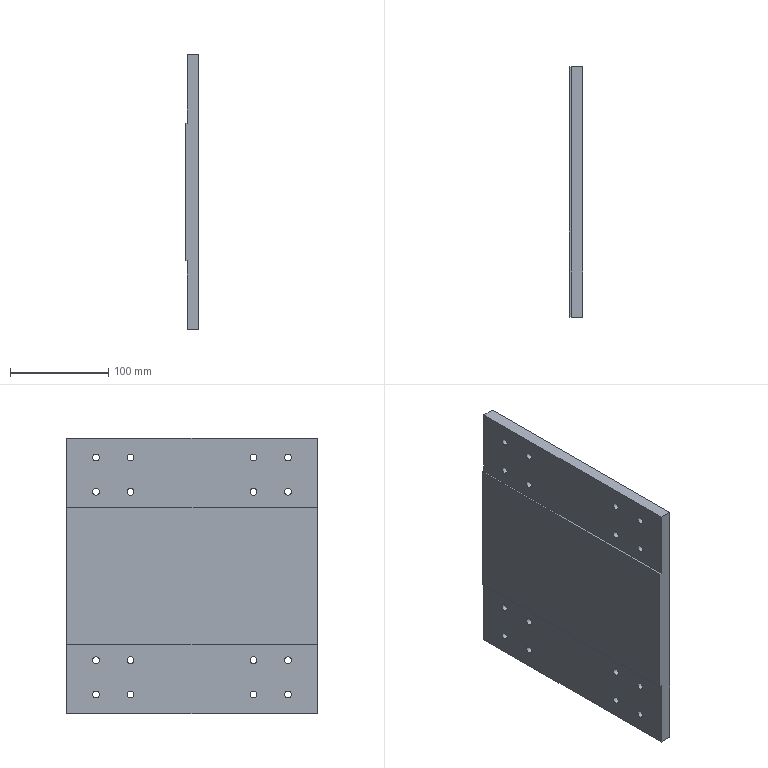Part | SolidWorks | features Extrusion 1, ICE 1 | 1 solid | 42 faces | box 14 x 255 x 280 mm | volume 920811 mm3 | cylinder 32 | plane 10 | commonest cylinder face diameters 7 x32
STEP:
#1=CARTESIAN_POINT('',(14.,62.5,-82.));
#2=VERTEX_POINT('',#1);
#3=CARTESIAN_POINT('',(14.,62.5,-89.));
#4=VERTEX_POINT('',#3);
#5=CARTESIAN_POINT('',(14.,62.5,-85.5));
#6=DIRECTION('',(1.,0.,0.));
#7=DIRECTION('',(0.,0.,-1.));
#8=AXIS2_PLACEMENT_3D('',#5,#6,#7);
#9=CIRCLE('',#8,3.5);
#10=EDGE_CURVE('',#2,#4,#9,.T.);
#11=ORIENTED_EDGE('',*,*,#10,.T.);
#12=CARTESIAN_POINT('',(2.,62.5,-89.));
#13=VERTEX_POINT('',#12);
#14=CARTESIAN_POINT('',(14.,62.5,-89.));
#15=DIRECTION('',(-1.,0.,0.));
#16=VECTOR('',#15,1000.);
#17=LINE('',#14,#16);
#18=EDGE_CURVE('',#4,#13,#17,.T.);
#19=ORIENTED_EDGE('',*,*,#18,.T.);
#20=CARTESIAN_POINT('',(2.,62.5,-82.));
#21=VERTEX_POINT('',#20);
#22=CARTESIAN_POINT('',(2.,62.5,-85.5));
#23=DIRECTION('',(-1.,0.,0.));
#24=DIRECTION('',(0.,0.,1.));
#25=AXIS2_PLACEMENT_3D('',#22,#23,#24);
#26=CIRCLE('',#25,3.5);
#27=EDGE_CURVE('',#13,#21,#26,.T.);
#28=ORIENTED_EDGE('',*,*,#27,.T.);
#29=CARTESIAN_POINT('',(14.,62.5,-82.));
#30=DIRECTION('',(-1.,0.,0.));
#31=VECTOR('',#30,1000.);
#32=LINE('',#29,#31);
#33=EDGE_CURVE('',#2,#21,#32,.T.);
#34=ORIENTED_EDGE('',*,*,#33,.F.);
#35=EDGE_LOOP('',(#11,#19,#28,#34));
#36=FACE_OUTER_BOUND('',#35,.T.);
#37=CARTESIAN_POINT('',(14.,62.5,-85.5));
#38=DIRECTION('',(-1.,0.,0.));
#39=DIRECTION('',(0.,0.,1.));
#40=AXIS2_PLACEMENT_3D('',#37,#38,#39);
#41=CYLINDRICAL_SURFACE('',#40,3.5);
#42=ADVANCED_FACE('',(#36),#41,.F.);
#43=CARTESIAN_POINT('',(14.,62.5,-117.));
#44=VERTEX_POINT('',#43);
#45=CARTESIAN_POINT('',(14.,62.5,-124.));
#46=VERTEX_POINT('',#45);
#47=CARTESIAN_POINT('',(14.,62.5,-120.5));
#48=DIRECTION('',(1.,0.,0.));
#49=DIRECTION('',(0.,0.,-1.));
#50=AXIS2_PLACEMENT_3D('',#47,#48,#49);
#51=CIRCLE('',#50,3.5);
#52=EDGE_CURVE('',#44,#46,#51,.T.);
#53=ORIENTED_EDGE('',*,*,#52,.T.);
#54=CARTESIAN_POINT('',(2.,62.5,-124.));
#55=VERTEX_POINT('',#54);
#56=CARTESIAN_POINT('',(14.,62.5,-124.));
#57=DIRECTION('',(-1.,0.,0.));
#58=VECTOR('',#57,1000.);
#59=LINE('',#56,#58);
#60=EDGE_CURVE('',#46,#55,#59,.T.);
#61=ORIENTED_EDGE('',*,*,#60,.T.);
#62=CARTESIAN_POINT('',(2.,62.5,-117.));
#63=VERTEX_POINT('',#62);
#64=CARTESIAN_POINT('',(2.,62.5,-120.5));
#65=DIRECTION('',(-1.,0.,0.));
#66=DIRECTION('',(0.,0.,1.));
#67=AXIS2_PLACEMENT_3D('',#64,#65,#66);
#68=CIRCLE('',#67,3.5);
#69=EDGE_CURVE('',#55,#63,#68,.T.);
#70=ORIENTED_EDGE('',*,*,#69,.T.);
#71=CARTESIAN_POINT('',(14.,62.5,-117.));
#72=DIRECTION('',(-1.,0.,0.));
#73=VECTOR('',#72,1000.);
#74=LINE('',#71,#73);
#75=EDGE_CURVE('',#44,#63,#74,.T.);
#76=ORIENTED_EDGE('',*,*,#75,.F.);
#77=EDGE_LOOP('',(#53,#61,#70,#76));
#78=FACE_OUTER_BOUND('',#77,.T.);
#79=CARTESIAN_POINT('',(14.,62.5,-120.5));
#80=DIRECTION('',(-1.,0.,0.));
#81=DIRECTION('',(0.,0.,1.));
#82=AXIS2_PLACEMENT_3D('',#79,#80,#81);
#83=CYLINDRICAL_SURFACE('',#82,3.5);
#84=ADVANCED_FACE('',(#78),#83,.F.);
#85=CARTESIAN_POINT('',(14.,-97.5,-117.));
#86=VERTEX_POINT('',#85);
#87=CARTESIAN_POINT('',(14.,-97.5,-124.));
#88=VERTEX_POINT('',#87);
#89=CARTESIAN_POINT('',(14.,-97.5,-120.5));
#90=DIRECTION('',(1.,0.,0.));
#91=DIRECTION('',(0.,0.,-1.));
#92=AXIS2_PLACEMENT_3D('',#89,#90,#91);
#93=CIRCLE('',#92,3.5);
#94=EDGE_CURVE('',#86,#88,#93,.T.);
#95=ORIENTED_EDGE('',*,*,#94,.T.);
#96=CARTESIAN_POINT('',(2.,-97.5,-124.));
#97=VERTEX_POINT('',#96);
#98=CARTESIAN_POINT('',(14.,-97.5,-124.));
#99=DIRECTION('',(-1.,0.,0.));
#100=VECTOR('',#99,1000.);
#101=LINE('',#98,#100);
#102=EDGE_CURVE('',#88,#97,#101,.T.);
#103=ORIENTED_EDGE('',*,*,#102,.T.);
#104=CARTESIAN_POINT('',(2.,-97.5,-117.));
#105=VERTEX_POINT('',#104);
#106=CARTESIAN_POINT('',(2.,-97.5,-120.5));
#107=DIRECTION('',(-1.,0.,0.));
#108=DIRECTION('',(0.,0.,1.));
#109=AXIS2_PLACEMENT_3D('',#106,#107,#108);
#110=CIRCLE('',#109,3.5);
#111=EDGE_CURVE('',#97,#105,#110,.T.);
#112=ORIENTED_EDGE('',*,*,#111,.T.);
#113=CARTESIAN_POINT('',(14.,-97.5,-117.));
#114=DIRECTION('',(-1.,0.,0.));
#115=VECTOR('',#114,1000.);
#116=LINE('',#113,#115);
#117=EDGE_CURVE('',#86,#105,#116,.T.);
#118=ORIENTED_EDGE('',*,*,#117,.F.);
#119=EDGE_LOOP('',(#95,#103,#112,#118));
#120=FACE_OUTER_BOUND('',#119,.T.);
#121=CARTESIAN_POINT('',(14.,-97.5,-120.5));
#122=DIRECTION('',(-1.,0.,0.));
#123=DIRECTION('',(0.,0.,1.));
#124=AXIS2_PLACEMENT_3D('',#121,#122,#123);
#125=CYLINDRICAL_SURFACE('',#124,3.5);
#126=ADVANCED_FACE('',(#120),#125,.F.);
#127=CARTESIAN_POINT('',(14.,-97.5,-82.));
#128=VERTEX_POINT('',#127);
#129=CARTESIAN_POINT('',(14.,-97.5,-89.));
#130=VERTEX_POINT('',#129);
#131=CARTESIAN_POINT('',(14.,-97.5,-85.5));
#132=DIRECTION('',(1.,0.,0.));
#133=DIRECTION('',(0.,0.,-1.));
#134=AXIS2_PLACEMENT_3D('',#131,#132,#133);
#135=CIRCLE('',#134,3.5);
#136=EDGE_CURVE('',#128,#130,#135,.T.);
#137=ORIENTED_EDGE('',*,*,#136,.T.);
#138=CARTESIAN_POINT('',(2.,-97.5,-89.));
#139=VERTEX_POINT('',#138);
#140=CARTESIAN_POINT('',(14.,-97.5,-89.));
#141=DIRECTION('',(-1.,0.,0.));
#142=VECTOR('',#141,1000.);
#143=LINE('',#140,#142);
#144=EDGE_CURVE('',#130,#139,#143,.T.);
#145=ORIENTED_EDGE('',*,*,#144,.T.);
#146=CARTESIAN_POINT('',(2.,-97.5,-82.));
#147=VERTEX_POINT('',#146);
#148=CARTESIAN_POINT('',(2.,-97.5,-85.5));
#149=DIRECTION('',(-1.,0.,0.));
#150=DIRECTION('',(0.,0.,1.));
#151=AXIS2_PLACEMENT_3D('',#148,#149,#150);
#152=CIRCLE('',#151,3.5);
#153=EDGE_CURVE('',#139,#147,#152,.T.);
#154=ORIENTED_EDGE('',*,*,#153,.T.);
#155=CARTESIAN_POINT('',(14.,-97.5,-82.));
#156=DIRECTION('',(-1.,0.,0.));
#157=VECTOR('',#156,1000.);
#158=LINE('',#155,#157);
#159=EDGE_CURVE('',#128,#147,#158,.T.);
#160=ORIENTED_EDGE('',*,*,#159,.F.);
#161=EDGE_LOOP('',(#137,#145,#154,#160));
#162=FACE_OUTER_BOUND('',#161,.T.);
#163=CARTESIAN_POINT('',(14.,-97.5,-85.5));
#164=DIRECTION('',(-1.,0.,0.));
#165=DIRECTION('',(0.,0.,1.));
#166=AXIS2_PLACEMENT_3D('',#163,#164,#165);
#167=CYLINDRICAL_SURFACE('',#166,3.5);
#168=ADVANCED_FACE('',(#162),#167,.F.);
#169=CARTESIAN_POINT('',(14.,-62.5,-117.));
#170=VERTEX_POINT('',#169);
#171=CARTESIAN_POINT('',(14.,-62.5,-124.));
#172=VERTEX_POINT('',#171);
#173=CARTESIAN_POINT('',(14.,-62.5,-120.5));
#174=DIRECTION('',(1.,0.,0.));
#175=DIRECTION('',(0.,0.,-1.));
#176=AXIS2_PLACEMENT_3D('',#173,#174,#175);
#177=CIRCLE('',#176,3.5);
#178=EDGE_CURVE('',#170,#172,#177,.T.);
#179=ORIENTED_EDGE('',*,*,#178,.T.);
#180=CARTESIAN_POINT('',(2.,-62.5,-124.));
#181=VERTEX_POINT('',#180);
#182=CARTESIAN_POINT('',(14.,-62.5,-124.));
#183=DIRECTION('',(-1.,0.,0.));
#184=VECTOR('',#183,1000.);
#185=LINE('',#182,#184);
#186=EDGE_CURVE('',#172,#181,#185,.T.);
#187=ORIENTED_EDGE('',*,*,#186,.T.);
#188=CARTESIAN_POINT('',(2.,-62.5,-117.));
#189=VERTEX_POINT('',#188);
#190=CARTESIAN_POINT('',(2.,-62.5,-120.5));
#191=DIRECTION('',(-1.,0.,0.));
#192=DIRECTION('',(0.,0.,1.));
#193=AXIS2_PLACEMENT_3D('',#190,#191,#192);
#194=CIRCLE('',#193,3.5);
#195=EDGE_CURVE('',#181,#189,#194,.T.);
#196=ORIENTED_EDGE('',*,*,#195,.T.);
#197=CARTESIAN_POINT('',(14.,-62.5,-117.));
#198=DIRECTION('',(-1.,0.,0.));
#199=VECTOR('',#198,1000.);
#200=LINE('',#197,#199);
#201=EDGE_CURVE('',#170,#189,#200,.T.);
#202=ORIENTED_EDGE('',*,*,#201,.F.);
#203=EDGE_LOOP('',(#179,#187,#196,#202));
#204=FACE_OUTER_BOUND('',#203,.T.);
#205=CARTESIAN_POINT('',(14.,-62.5,-120.5));
#206=DIRECTION('',(-1.,0.,0.));
#207=DIRECTION('',(0.,0.,1.));
#208=AXIS2_PLACEMENT_3D('',#205,#206,#207);
#209=CYLINDRICAL_SURFACE('',#208,3.5);
#210=ADVANCED_FACE('',(#204),#209,.F.);
#211=CARTESIAN_POINT('',(14.,-62.5,-82.));
#212=VERTEX_POINT('',#211);
#213=CARTESIAN_POINT('',(14.,-62.5,-89.));
#214=VERTEX_POINT('',#213);
#215=CARTESIAN_POINT('',(14.,-62.5,-85.5));
#216=DIRECTION('',(1.,0.,0.));
#217=DIRECTION('',(0.,0.,-1.));
#218=AXIS2_PLACEMENT_3D('',#215,#216,#217);
#219=CIRCLE('',#218,3.5);
#220=EDGE_CURVE('',#212,#214,#219,.T.);
#221=ORIENTED_EDGE('',*,*,#220,.T.);
#222=CARTESIAN_POINT('',(2.,-62.5,-89.));
#223=VERTEX_POINT('',#222);
#224=CARTESIAN_POINT('',(14.,-62.5,-89.));
#225=DIRECTION('',(-1.,0.,0.));
#226=VECTOR('',#225,1000.);
#227=LINE('',#224,#226);
#228=EDGE_CURVE('',#214,#223,#227,.T.);
#229=ORIENTED_EDGE('',*,*,#228,.T.);
#230=CARTESIAN_POINT('',(2.,-62.5,-82.));
#231=VERTEX_POINT('',#230);
#232=CARTESIAN_POINT('',(2.,-62.5,-85.5));
#233=DIRECTION('',(-1.,0.,0.));
#234=DIRECTION('',(0.,0.,1.));
#235=AXIS2_PLACEMENT_3D('',#232,#233,#234);
#236=CIRCLE('',#235,3.5);
#237=EDGE_CURVE('',#223,#231,#236,.T.);
#238=ORIENTED_EDGE('',*,*,#237,.T.);
#239=CARTESIAN_POINT('',(14.,-62.5,-82.));
#240=DIRECTION('',(-1.,0.,0.));
#241=VECTOR('',#240,1000.);
#242=LINE('',#239,#241);
#243=EDGE_CURVE('',#212,#231,#242,.T.);
#244=ORIENTED_EDGE('',*,*,#243,.F.);
#245=EDGE_LOOP('',(#221,#229,#238,#244));
#246=FACE_OUTER_BOUND('',#245,.T.);
#247=CARTESIAN_POINT('',(14.,-62.5,-85.5));
#248=DIRECTION('',(-1.,0.,0.));
#249=DIRECTION('',(0.,0.,1.));
#250=AXIS2_PLACEMENT_3D('',#247,#248,#249);
#251=CYLINDRICAL_SURFACE('',#250,3.5);
#252=ADVANCED_FACE('',(#246),#251,.F.);
#253=CARTESIAN_POINT('',(14.,97.5,-117.));
#254=VERTEX_POINT('',#253);
#255=CARTESIAN_POINT('',(14.,97.5,-124.));
#256=VERTEX_POINT('',#255);
#257=CARTESIAN_POINT('',(14.,97.5,-120.5));
#258=DIRECTION('',(1.,0.,0.));
#259=DIRECTION('',(0.,0.,-1.));
#260=AXIS2_PLACEMENT_3D('',#257,#258,#259);
#261=CIRCLE('',#260,3.5);
#262=EDGE_CURVE('',#254,#256,#261,.T.);
#263=ORIENTED_EDGE('',*,*,#262,.T.);
#264=CARTESIAN_POINT('',(2.,97.5,-124.));
#265=VERTEX_POINT('',#264);
#266=CARTESIAN_POINT('',(14.,97.5,-124.));
#267=DIRECTION('',(-1.,0.,0.));
#268=VECTOR('',#267,1000.);
#269=LINE('',#266,#268);
#270=EDGE_CURVE('',#256,#265,#269,.T.);
#271=ORIENTED_EDGE('',*,*,#270,.T.);
#272=CARTESIAN_POINT('',(2.,97.5,-117.));
#273=VERTEX_POINT('',#272);
#274=CARTESIAN_POINT('',(2.,97.5,-120.5));
#275=DIRECTION('',(-1.,0.,0.));
#276=DIRECTION('',(0.,0.,1.));
#277=AXIS2_PLACEMENT_3D('',#274,#275,#276);
#278=CIRCLE('',#277,3.5);
#279=EDGE_CURVE('',#265,#273,#278,.T.);
#280=ORIENTED_EDGE('',*,*,#279,.T.);
#281=CARTESIAN_POINT('',(14.,97.5,-117.));
#282=DIRECTION('',(-1.,0.,0.));
#283=VECTOR('',#282,1000.);
#284=LINE('',#281,#283);
#285=EDGE_CURVE('',#254,#273,#284,.T.);
#286=ORIENTED_EDGE('',*,*,#285,.F.);
#287=EDGE_LOOP('',(#263,#271,#280,#286));
#288=FACE_OUTER_BOUND('',#287,.T.);
#289=CARTESIAN_POINT('',(14.,97.5,-120.5));
#290=DIRECTION('',(-1.,0.,0.));
#291=DIRECTION('',(0.,0.,1.));
#292=AXIS2_PLACEMENT_3D('',#289,#290,#291);
#293=CYLINDRICAL_SURFACE('',#292,3.5);
#294=ADVANCED_FACE('',(#288),#293,.F.);
#295=CARTESIAN_POINT('',(14.,97.5,-82.));
#296=VERTEX_POINT('',#295);
#297=CARTESIAN_POINT('',(14.,97.5,-89.));
#298=VERTEX_POINT('',#297);
#299=CARTESIAN_POINT('',(14.,97.5,-85.5));
#300=DIRECTION('',(1.,0.,0.));
#301=DIRECTION('',(0.,0.,-1.));
#302=AXIS2_PLACEMENT_3D('',#299,#300,#301);
#303=CIRCLE('',#302,3.5);
#304=EDGE_CURVE('',#296,#298,#303,.T.);
#305=ORIENTED_EDGE('',*,*,#304,.T.);
#306=CARTESIAN_POINT('',(2.,97.5,-89.));
#307=VERTEX_POINT('',#306);
#308=CARTESIAN_POINT('',(14.,97.5,-89.));
#309=DIRECTION('',(-1.,0.,0.));
#310=VECTOR('',#309,1000.);
#311=LINE('',#308,#310);
#312=EDGE_CURVE('',#298,#307,#311,.T.);
#313=ORIENTED_EDGE('',*,*,#312,.T.);
#314=CARTESIAN_POINT('',(2.,97.5,-82.));
#315=VERTEX_POINT('',#314);
#316=CARTESIAN_POINT('',(2.,97.5,-85.5));
#317=DIRECTION('',(-1.,0.,0.));
#318=DIRECTION('',(0.,0.,1.));
#319=AXIS2_PLACEMENT_3D('',#316,#317,#318);
#320=CIRCLE('',#319,3.5);
#321=EDGE_CURVE('',#307,#315,#320,.T.);
#322=ORIENTED_EDGE('',*,*,#321,.T.);
#323=CARTESIAN_POINT('',(14.,97.5,-82.));
#324=DIRECTION('',(-1.,0.,0.));
#325=VECTOR('',#324,1000.);
#326=LINE('',#323,#325);
#327=EDGE_CURVE('',#296,#315,#326,.T.);
#328=ORIENTED_EDGE('',*,*,#327,.F.);
#329=EDGE_LOOP('',(#305,#313,#322,#328));
#330=FACE_OUTER_BOUND('',#329,.T.);
#331=CARTESIAN_POINT('',(14.,97.5,-85.5));
#332=DIRECTION('',(-1.,0.,0.));
#333=DIRECTION('',(0.,0.,1.));
#334=AXIS2_PLACEMENT_3D('',#331,#332,#333);
#335=CYLINDRICAL_SURFACE('',#334,3.5);
#336=ADVANCED_FACE('',(#330),#335,.F.);
#337=CARTESIAN_POINT('',(14.,-62.5,89.));
#338=VERTEX_POINT('',#337);
#339=CARTESIAN_POINT('',(14.,-62.5,82.));
#340=VERTEX_POINT('',#339);
#341=CARTESIAN_POINT('',(14.,-62.5,85.5));
#342=DIRECTION('',(1.,0.,0.));
#343=DIRECTION('',(0.,0.,-1.));
#344=AXIS2_PLACEMENT_3D('',#341,#342,#343);
#345=CIRCLE('',#344,3.5);
#346=EDGE_CURVE('',#338,#340,#345,.T.);
#347=ORIENTED_EDGE('',*,*,#346,.T.);
#348=CARTESIAN_POINT('',(2.,-62.5,82.));
#349=VERTEX_POINT('',#348);
#350=CARTESIAN_POINT('',(14.,-62.5,82.));
#351=DIRECTION('',(-1.,0.,0.));
#352=VECTOR('',#351,1000.);
#353=LINE('',#350,#352);
#354=EDGE_CURVE('',#340,#349,#353,.T.);
#355=ORIENTED_EDGE('',*,*,#354,.T.);
#356=CARTESIAN_POINT('',(2.,-62.5,89.));
#357=VERTEX_POINT('',#356);
#358=CARTESIAN_POINT('',(2.,-62.5,85.5));
#359=DIRECTION('',(-1.,0.,0.));
#360=DIRECTION('',(0.,0.,1.));
#361=AXIS2_PLACEMENT_3D('',#358,#359,#360);
#362=CIRCLE('',#361,3.5);
#363=EDGE_CURVE('',#349,#357,#362,.T.);
#364=ORIENTED_EDGE('',*,*,#363,.T.);
#365=CARTESIAN_POINT('',(14.,-62.5,89.));
#366=DIRECTION('',(-1.,0.,0.));
#367=VECTOR('',#366,1000.);
#368=LINE('',#365,#367);
#369=EDGE_CURVE('',#338,#357,#368,.T.);
#370=ORIENTED_EDGE('',*,*,#369,.F.);
#371=EDGE_LOOP('',(#347,#355,#364,#370));
#372=FACE_OUTER_BOUND('',#371,.T.);
#373=CARTESIAN_POINT('',(14.,-62.5,85.5));
#374=DIRECTION('',(-1.,0.,0.));
#375=DIRECTION('',(0.,0.,1.));
#376=AXIS2_PLACEMENT_3D('',#373,#374,#375);
#377=CYLINDRICAL_SURFACE('',#376,3.5);
#378=ADVANCED_FACE('',(#372),#377,.F.);
#379=CARTESIAN_POINT('',(14.,-62.5,124.));
#380=VERTEX_POINT('',#379);
#381=CARTESIAN_POINT('',(14.,-62.5,117.));
#382=VERTEX_POINT('',#381);
#383=CARTESIAN_POINT('',(14.,-62.5,120.5));
#384=DIRECTION('',(1.,0.,0.));
#385=DIRECTION('',(0.,0.,-1.));
#386=AXIS2_PLACEMENT_3D('',#383,#384,#385);
#387=CIRCLE('',#386,3.5);
#388=EDGE_CURVE('',#380,#382,#387,.T.);
#389=ORIENTED_EDGE('',*,*,#388,.T.);
#390=CARTESIAN_POINT('',(2.,-62.5,117.));
#391=VERTEX_POINT('',#390);
#392=CARTESIAN_POINT('',(14.,-62.5,117.));
#393=DIRECTION('',(-1.,0.,0.));
#394=VECTOR('',#393,1000.);
#395=LINE('',#392,#394);
#396=EDGE_CURVE('',#382,#391,#395,.T.);
#397=ORIENTED_EDGE('',*,*,#396,.T.);
#398=CARTESIAN_POINT('',(2.,-62.5,124.));
#399=VERTEX_POINT('',#398);
#400=CARTESIAN_POINT('',(2.,-62.5,120.5));
#401=DIRECTION('',(-1.,0.,0.));
#402=DIRECTION('',(0.,0.,1.));
#403=AXIS2_PLACEMENT_3D('',#400,#401,#402);
#404=CIRCLE('',#403,3.5);
#405=EDGE_CURVE('',#391,#399,#404,.T.);
#406=ORIENTED_EDGE('',*,*,#405,.T.);
#407=CARTESIAN_POINT('',(14.,-62.5,124.));
#408=DIRECTION('',(-1.,0.,0.));
#409=VECTOR('',#408,1000.);
#410=LINE('',#407,#409);
#411=EDGE_CURVE('',#380,#399,#410,.T.);
#412=ORIENTED_EDGE('',*,*,#411,.F.);
#413=EDGE_LOOP('',(#389,#397,#406,#412));
#414=FACE_OUTER_BOUND('',#413,.T.);
#415=CARTESIAN_POINT('',(14.,-62.5,120.5));
#416=DIRECTION('',(-1.,0.,0.));
#417=DIRECTION('',(0.,0.,1.));
#418=AXIS2_PLACEMENT_3D('',#415,#416,#417);
#419=CYLINDRICAL_SURFACE('',#418,3.5);
#420=ADVANCED_FACE('',(#414),#419,.F.);
#421=CARTESIAN_POINT('',(14.,62.5,89.));
#422=VERTEX_POINT('',#421);
#423=CARTESIAN_POINT('',(14.,62.5,82.));
#424=VERTEX_POINT('',#423);
#425=CARTESIAN_POINT('',(14.,62.5,85.5));
#426=DIRECTION('',(1.,0.,0.));
#427=DIRECTION('',(0.,0.,-1.));
#428=AXIS2_PLACEMENT_3D('',#425,#426,#427);
#429=CIRCLE('',#428,3.5);
#430=EDGE_CURVE('',#422,#424,#429,.T.);
#431=ORIENTED_EDGE('',*,*,#430,.T.);
#432=CARTESIAN_POINT('',(2.,62.5,82.));
#433=VERTEX_POINT('',#432);
#434=CARTESIAN_POINT('',(14.,62.5,82.));
#435=DIRECTION('',(-1.,0.,0.));
#436=VECTOR('',#435,1000.);
#437=LINE('',#434,#436);
#438=EDGE_CURVE('',#424,#433,#437,.T.);
#439=ORIENTED_EDGE('',*,*,#438,.T.);
#440=CARTESIAN_POINT('',(2.,62.5,89.));
#441=VERTEX_POINT('',#440);
#442=CARTESIAN_POINT('',(2.,62.5,85.5));
#443=DIRECTION('',(-1.,0.,0.));
#444=DIRECTION('',(0.,0.,1.));
#445=AXIS2_PLACEMENT_3D('',#442,#443,#444);
#446=CIRCLE('',#445,3.5);
#447=EDGE_CURVE('',#433,#441,#446,.T.);
#448=ORIENTED_EDGE('',*,*,#447,.T.);
#449=CARTESIAN_POINT('',(14.,62.5,89.));
#450=DIRECTION('',(-1.,0.,0.));
#451=VECTOR('',#450,1000.);
#452=LINE('',#449,#451);
#453=EDGE_CURVE('',#422,#441,#452,.T.);
#454=ORIENTED_EDGE('',*,*,#453,.F.);
#455=EDGE_LOOP('',(#431,#439,#448,#454));
#456=FACE_OUTER_BOUND('',#455,.T.);
#457=CARTESIAN_POINT('',(14.,62.5,85.5));
#458=DIRECTION('',(-1.,0.,0.));
#459=DIRECTION('',(0.,0.,1.));
#460=AXIS2_PLACEMENT_3D('',#457,#458,#459);
#461=CYLINDRICAL_SURFACE('',#460,3.5);
#462=ADVANCED_FACE('',(#456),#461,.F.);
#463=CARTESIAN_POINT('',(14.,62.5,124.));
#464=VERTEX_POINT('',#463);
#465=CARTESIAN_POINT('',(14.,62.5,117.));
#466=VERTEX_POINT('',#465);
#467=CARTESIAN_POINT('',(14.,62.5,120.5));
#468=DIRECTION('',(1.,0.,0.));
#469=DIRECTION('',(0.,0.,-1.));
#470=AXIS2_PLACEMENT_3D('',#467,#468,#469);
#471=CIRCLE('',#470,3.5);
#472=EDGE_CURVE('',#464,#466,#471,.T.);
#473=ORIENTED_EDGE('',*,*,#472,.T.);
#474=CARTESIAN_POINT('',(2.,62.5,117.));
#475=VERTEX_POINT('',#474);
#476=CARTESIAN_POINT('',(14.,62.5,117.));
#477=DIRECTION('',(-1.,0.,0.));
#478=VECTOR('',#477,1000.);
#479=LINE('',#476,#478);
#480=EDGE_CURVE('',#466,#475,#479,.T.);
#481=ORIENTED_EDGE('',*,*,#480,.T.);
#482=CARTESIAN_POINT('',(2.,62.5,124.));
#483=VERTEX_POINT('',#482);
#484=CARTESIAN_POINT('',(2.,62.5,120.5));
#485=DIRECTION('',(-1.,0.,0.));
#486=DIRECTION('',(0.,0.,1.));
#487=AXIS2_PLACEMENT_3D('',#484,#485,#486);
#488=CIRCLE('',#487,3.5);
#489=EDGE_CURVE('',#475,#483,#488,.T.);
#490=ORIENTED_EDGE('',*,*,#489,.T.);
#491=CARTESIAN_POINT('',(14.,62.5,124.));
#492=DIRECTION('',(-1.,0.,0.));
#493=VECTOR('',#492,1000.);
#494=LINE('',#491,#493);
#495=EDGE_CURVE('',#464,#483,#494,.T.);
#496=ORIENTED_EDGE('',*,*,#495,.F.);
#497=EDGE_LOOP('',(#473,#481,#490,#496));
#498=FACE_OUTER_BOUND('',#497,.T.);
#499=CARTESIAN_POINT('',(14.,62.5,120.5));
#500=DIRECTION('',(-1.,0.,0.));
#501=DIRECTION('',(0.,0.,1.));
#502=AXIS2_PLACEMENT_3D('',#499,#500,#501);
#503=CYLINDRICAL_SURFACE('',#502,3.5);
#504=ADVANCED_FACE('',(#498),#503,.F.);
#505=CARTESIAN_POINT('',(14.,-97.5,89.));
#506=VERTEX_POINT('',#505);
#507=CARTESIAN_POINT('',(14.,-97.5,82.));
#508=VERTEX_POINT('',#507);
#509=CARTESIAN_POINT('',(14.,-97.5,85.5));
#510=DIRECTION('',(1.,0.,0.));
#511=DIRECTION('',(0.,0.,-1.));
#512=AXIS2_PLACEMENT_3D('',#509,#510,#511);
#513=CIRCLE('',#512,3.5);
#514=EDGE_CURVE('',#506,#508,#513,.T.);
#515=ORIENTED_EDGE('',*,*,#514,.T.);
#516=CARTESIAN_POINT('',(2.,-97.5,82.));
#517=VERTEX_POINT('',#516);
#518=CARTESIAN_POINT('',(14.,-97.5,82.));
#519=DIRECTION('',(-1.,0.,0.));
#520=VECTOR('',#519,1000.);
#521=LINE('',#518,#520);
#522=EDGE_CURVE('',#508,#517,#521,.T.);
#523=ORIENTED_EDGE('',*,*,#522,.T.);
#524=CARTESIAN_POINT('',(2.,-97.5,89.));
#525=VERTEX_POINT('',#524);
#526=CARTESIAN_POINT('',(2.,-97.5,85.5));
#527=DIRECTION('',(-1.,0.,0.));
#528=DIRECTION('',(0.,0.,1.));
#529=AXIS2_PLACEMENT_3D('',#526,#527,#528);
#530=CIRCLE('',#529,3.5);
#531=EDGE_CURVE('',#517,#525,#530,.T.);
#532=ORIENTED_EDGE('',*,*,#531,.T.);
#533=CARTESIAN_POINT('',(14.,-97.5,89.));
#534=DIRECTION('',(-1.,0.,0.));
#535=VECTOR('',#534,1000.);
#536=LINE('',#533,#535);
#537=EDGE_CURVE('',#506,#525,#536,.T.);
#538=ORIENTED_EDGE('',*,*,#537,.F.);
#539=EDGE_LOOP('',(#515,#523,#532,#538));
#540=FACE_OUTER_BOUND('',#539,.T.);
#541=CARTESIAN_POINT('',(14.,-97.5,85.5));
#542=DIRECTION('',(-1.,0.,0.));
#543=DIRECTION('',(0.,0.,1.));
#544=AXIS2_PLACEMENT_3D('',#541,#542,#543);
#545=CYLINDRICAL_SURFACE('',#544,3.5);
#546=ADVANCED_FACE('',(#540),#545,.F.);
#547=CARTESIAN_POINT('',(14.,-97.5,124.));
#548=VERTEX_POINT('',#547);
#549=CARTESIAN_POINT('',(14.,-97.5,117.));
#550=VERTEX_POINT('',#549);
#551=CARTESIAN_POINT('',(14.,-97.5,120.5));
#552=DIRECTION('',(1.,0.,0.));
#553=DIRECTION('',(0.,0.,-1.));
#554=AXIS2_PLACEMENT_3D('',#551,#552,#553);
#555=CIRCLE('',#554,3.5);
#556=EDGE_CURVE('',#548,#550,#555,.T.);
#557=ORIENTED_EDGE('',*,*,#556,.T.);
#558=CARTESIAN_POINT('',(2.,-97.5,117.));
#559=VERTEX_POINT('',#558);
#560=CARTESIAN_POINT('',(14.,-97.5,117.));
#561=DIRECTION('',(-1.,0.,0.));
#562=VECTOR('',#561,1000.);
#563=LINE('',#560,#562);
#564=EDGE_CURVE('',#550,#559,#563,.T.);
#565=ORIENTED_EDGE('',*,*,#564,.T.);
#566=CARTESIAN_POINT('',(2.,-97.5,124.));
#567=VERTEX_POINT('',#566);
#568=CARTESIAN_POINT('',(2.,-97.5,120.5));
#569=DIRECTION('',(-1.,0.,0.));
#570=DIRECTION('',(0.,0.,1.));
#571=AXIS2_PLACEMENT_3D('',#568,#569,#570);
#572=CIRCLE('',#571,3.5);
#573=EDGE_CURVE('',#559,#567,#572,.T.);
#574=ORIENTED_EDGE('',*,*,#573,.T.);
#575=CARTESIAN_POINT('',(14.,-97.5,124.));
#576=DIRECTION('',(-1.,0.,0.));
#577=VECTOR('',#576,1000.);
#578=LINE('',#575,#577);
#579=EDGE_CURVE('',#548,#567,#578,.T.);
#580=ORIENTED_EDGE('',*,*,#579,.F.);
#581=EDGE_LOOP('',(#557,#565,#574,#580));
#582=FACE_OUTER_BOUND('',#581,.T.);
#583=CARTESIAN_POINT('',(14.,-97.5,120.5));
#584=DIRECTION('',(-1.,0.,0.));
#585=DIRECTION('',(0.,0.,1.));
#586=AXIS2_PLACEMENT_3D('',#583,#584,#585);
#587=CYLINDRICAL_SURFACE('',#586,3.5);
#588=ADVANCED_FACE('',(#582),#587,.F.);
#589=CARTESIAN_POINT('',(14.,97.5,89.));
#590=VERTEX_POINT('',#589);
#591=CARTESIAN_POINT('',(14.,97.5,82.));
#592=VERTEX_POINT('',#591);
#593=CARTESIAN_POINT('',(14.,97.5,85.5));
#594=DIRECTION('',(1.,0.,0.));
#595=DIRECTION('',(0.,0.,-1.));
#596=AXIS2_PLACEMENT_3D('',#593,#594,#595);
#597=CIRCLE('',#596,3.5);
#598=EDGE_CURVE('',#590,#592,#597,.T.);
#599=ORIENTED_EDGE('',*,*,#598,.T.);
#600=CARTESIAN_POINT('',(2.,97.5,82.));
#601=VERTEX_POINT('',#600);
#602=CARTESIAN_POINT('',(14.,97.5,82.));
#603=DIRECTION('',(-1.,0.,0.));
#604=VECTOR('',#603,1000.);
#605=LINE('',#602,#604);
#606=EDGE_CURVE('',#592,#601,#605,.T.);
#607=ORIENTED_EDGE('',*,*,#606,.T.);
#608=CARTESIAN_POINT('',(2.,97.5,89.));
#609=VERTEX_POINT('',#608);
#610=CARTESIAN_POINT('',(2.,97.5,85.5));
#611=DIRECTION('',(-1.,0.,0.));
#612=DIRECTION('',(0.,0.,1.));
#613=AXIS2_PLACEMENT_3D('',#610,#611,#612);
#614=CIRCLE('',#613,3.5);
#615=EDGE_CURVE('',#601,#609,#614,.T.);
#616=ORIENTED_EDGE('',*,*,#615,.T.);
#617=CARTESIAN_POINT('',(14.,97.5,89.));
#618=DIRECTION('',(-1.,0.,0.));
#619=VECTOR('',#618,1000.);
#620=LINE('',#617,#619);
#621=EDGE_CURVE('',#590,#609,#620,.T.);
#622=ORIENTED_EDGE('',*,*,#621,.F.);
#623=EDGE_LOOP('',(#599,#607,#616,#622));
#624=FACE_OUTER_BOUND('',#623,.T.);
#625=CARTESIAN_POINT('',(14.,97.5,85.5));
#626=DIRECTION('',(-1.,0.,0.));
#627=DIRECTION('',(0.,0.,1.));
#628=AXIS2_PLACEMENT_3D('',#625,#626,#627);
#629=CYLINDRICAL_SURFACE('',#628,3.5);
#630=ADVANCED_FACE('',(#624),#629,.F.);
#631=CARTESIAN_POINT('',(14.,97.5,124.));
#632=VERTEX_POINT('',#631);
#633=CARTESIAN_POINT('',(14.,97.5,117.));
#634=VERTEX_POINT('',#633);
#635=CARTESIAN_POINT('',(14.,97.5,120.5));
#636=DIRECTION('',(1.,0.,0.));
#637=DIRECTION('',(0.,0.,-1.));
#638=AXIS2_PLACEMENT_3D('',#635,#636,#637);
#639=CIRCLE('',#638,3.5);
#640=EDGE_CURVE('',#632,#634,#639,.T.);
#641=ORIENTED_EDGE('',*,*,#640,.T.);
#642=CARTESIAN_POINT('',(2.,97.5,117.));
#643=VERTEX_POINT('',#642);
#644=CARTESIAN_POINT('',(14.,97.5,117.));
#645=DIRECTION('',(-1.,0.,0.));
#646=VECTOR('',#645,1000.);
#647=LINE('',#644,#646);
#648=EDGE_CURVE('',#634,#643,#647,.T.);
#649=ORIENTED_EDGE('',*,*,#648,.T.);
#650=CARTESIAN_POINT('',(2.,97.5,124.));
#651=VERTEX_POINT('',#650);
#652=CARTESIAN_POINT('',(2.,97.5,120.5));
#653=DIRECTION('',(-1.,0.,0.));
#654=DIRECTION('',(0.,0.,1.));
#655=AXIS2_PLACEMENT_3D('',#652,#653,#654);
#656=CIRCLE('',#655,3.5);
#657=EDGE_CURVE('',#643,#651,#656,.T.);
#658=ORIENTED_EDGE('',*,*,#657,.T.);
#659=CARTESIAN_POINT('',(14.,97.5,124.));
#660=DIRECTION('',(-1.,0.,0.));
#661=VECTOR('',#660,1000.);
#662=LINE('',#659,#661);
#663=EDGE_CURVE('',#632,#651,#662,.T.);
#664=ORIENTED_EDGE('',*,*,#663,.F.);
#665=EDGE_LOOP('',(#641,#649,#658,#664));
#666=FACE_OUTER_BOUND('',#665,.T.);
#667=CARTESIAN_POINT('',(14.,97.5,120.5));
#668=DIRECTION('',(-1.,0.,0.));
#669=DIRECTION('',(0.,0.,1.));
#670=AXIS2_PLACEMENT_3D('',#667,#668,#669);
#671=CYLINDRICAL_SURFACE('',#670,3.5);
#672=ADVANCED_FACE('',(#666),#671,.F.);
#673=CARTESIAN_POINT('',(2.,127.5,-140.));
#674=VERTEX_POINT('',#673);
#675=CARTESIAN_POINT('',(2.,-127.5,-140.));
#676=VERTEX_POINT('',#675);
#677=CARTESIAN_POINT('',(2.,127.5,-140.));
#678=DIRECTION('',(0.,-1.,0.));
#679=VECTOR('',#678,1000.);
#680=LINE('',#677,#679);
#681=EDGE_CURVE('',#674,#676,#680,.T.);
#682=ORIENTED_EDGE('',*,*,#681,.F.);
#683=CARTESIAN_POINT('',(14.,127.5,-140.));
#684=VERTEX_POINT('',#683);
#685=CARTESIAN_POINT('',(14.,127.5,-140.));
#686=DIRECTION('',(-1.,0.,0.));
#687=VECTOR('',#686,1000.);
#688=LINE('',#685,#687);
#689=EDGE_CURVE('',#684,#674,#688,.T.);
#690=ORIENTED_EDGE('',*,*,#689,.F.);
#691=CARTESIAN_POINT('',(14.,-127.5,-140.));
#692=VERTEX_POINT('',#691);
#693=CARTESIAN_POINT('',(14.,-127.5,-140.));
#694=DIRECTION('',(0.,1.,0.));
#695=VECTOR('',#694,1000.);
#696=LINE('',#693,#695);
#697=EDGE_CURVE('',#692,#684,#696,.T.);
#698=ORIENTED_EDGE('',*,*,#697,.F.);
#699=CARTESIAN_POINT('',(14.,-127.5,-140.));
#700=DIRECTION('',(-1.,0.,0.));
#701=VECTOR('',#700,1000.);
#702=LINE('',#699,#701);
#703=EDGE_CURVE('',#692,#676,#702,.T.);
#704=ORIENTED_EDGE('',*,*,#703,.T.);
#705=EDGE_LOOP('',(#682,#690,#698,#704));
#706=FACE_OUTER_BOUND('',#705,.T.);
#707=CARTESIAN_POINT('',(14.,-127.5,-140.));
#708=DIRECTION('',(0.,0.,1.));
#709=DIRECTION('',(1.,0.,0.));
#710=AXIS2_PLACEMENT_3D('',#707,#708,#709);
#711=PLANE('',#710);
#712=ADVANCED_FACE('',(#706),#711,.F.);
#713=CARTESIAN_POINT('',(2.,-127.5,140.));
#714=VERTEX_POINT('',#713);
#715=CARTESIAN_POINT('',(2.,127.5,140.));
#716=VERTEX_POINT('',#715);
#717=CARTESIAN_POINT('',(2.,127.5,140.));
#718=DIRECTION('',(0.,1.,0.));
#719=VECTOR('',#718,1000.);
#720=LINE('',#717,#719);
#721=EDGE_CURVE('',#714,#716,#720,.T.);
#722=ORIENTED_EDGE('',*,*,#721,.F.);
#723=CARTESIAN_POINT('',(14.,-127.5,140.));
#724=VERTEX_POINT('',#723);
#725=CARTESIAN_POINT('',(14.,-127.5,140.));
#726=DIRECTION('',(-1.,0.,0.));
#727=VECTOR('',#726,1000.);
#728=LINE('',#725,#727);
#729=EDGE_CURVE('',#724,#714,#728,.T.);
#730=ORIENTED_EDGE('',*,*,#729,.F.);
#731=CARTESIAN_POINT('',(14.,127.5,140.));
#732=VERTEX_POINT('',#731);
#733=CARTESIAN_POINT('',(14.,-127.5,140.));
#734=DIRECTION('',(0.,-1.,0.));
#735=VECTOR('',#734,1000.);
#736=LINE('',#733,#735);
#737=EDGE_CURVE('',#732,#724,#736,.T.);
#738=ORIENTED_EDGE('',*,*,#737,.F.);
#739=CARTESIAN_POINT('',(14.,127.5,140.));
#740=DIRECTION('',(-1.,0.,0.));
#741=VECTOR('',#740,1000.);
#742=LINE('',#739,#741);
#743=EDGE_CURVE('',#732,#716,#742,.T.);
#744=ORIENTED_EDGE('',*,*,#743,.T.);
#745=EDGE_LOOP('',(#722,#730,#738,#744));
#746=FACE_OUTER_BOUND('',#745,.T.);
#747=CARTESIAN_POINT('',(14.,-127.5,140.));
#748=DIRECTION('',(0.,0.,-1.));
#749=DIRECTION('',(-1.,0.,0.));
#750=AXIS2_PLACEMENT_3D('',#747,#748,#749);
#751=PLANE('',#750);
#752=ADVANCED_FACE('',(#746),#751,.F.);
#753=ORIENTED_EDGE('',*,*,#648,.F.);
#754=CARTESIAN_POINT('',(14.,97.5,120.5));
#755=DIRECTION('',(1.,0.,0.));
#756=DIRECTION('',(0.,0.,-1.));
#757=AXIS2_PLACEMENT_3D('',#754,#755,#756);
#758=CIRCLE('',#757,3.5);
#759=EDGE_CURVE('',#634,#632,#758,.T.);
#760=ORIENTED_EDGE('',*,*,#759,.T.);
#761=ORIENTED_EDGE('',*,*,#663,.T.);
#762=CARTESIAN_POINT('',(2.,97.5,120.5));
#763=DIRECTION('',(-1.,0.,0.));
#764=DIRECTION('',(0.,0.,1.));
#765=AXIS2_PLACEMENT_3D('',#762,#763,#764);
#766=CIRCLE('',#765,3.5);
#767=EDGE_CURVE('',#651,#643,#766,.T.);
#768=ORIENTED_EDGE('',*,*,#767,.T.);
#769=EDGE_LOOP('',(#753,#760,#761,#768));
#770=FACE_OUTER_BOUND('',#769,.T.);
#771=CARTESIAN_POINT('',(14.,97.5,120.5));
#772=DIRECTION('',(-1.,0.,0.));
#773=DIRECTION('',(0.,0.,1.));
#774=AXIS2_PLACEMENT_3D('',#771,#772,#773);
#775=CYLINDRICAL_SURFACE('',#774,3.5);
#776=ADVANCED_FACE('',(#770),#775,.F.);
#777=ORIENTED_EDGE('',*,*,#606,.F.);
#778=CARTESIAN_POINT('',(14.,97.5,85.5));
#779=DIRECTION('',(1.,0.,0.));
#780=DIRECTION('',(0.,0.,-1.));
#781=AXIS2_PLACEMENT_3D('',#778,#779,#780);
#782=CIRCLE('',#781,3.5);
#783=EDGE_CURVE('',#592,#590,#782,.T.);
#784=ORIENTED_EDGE('',*,*,#783,.T.);
#785=ORIENTED_EDGE('',*,*,#621,.T.);
#786=CARTESIAN_POINT('',(2.,97.5,85.5));
#787=DIRECTION('',(-1.,0.,0.));
#788=DIRECTION('',(0.,0.,1.));
#789=AXIS2_PLACEMENT_3D('',#786,#787,#788);
#790=CIRCLE('',#789,3.5);
#791=EDGE_CURVE('',#609,#601,#790,.T.);
#792=ORIENTED_EDGE('',*,*,#791,.T.);
#793=EDGE_LOOP('',(#777,#784,#785,#792));
#794=FACE_OUTER_BOUND('',#793,.T.);
#795=CARTESIAN_POINT('',(14.,97.5,85.5));
#796=DIRECTION('',(-1.,0.,0.));
#797=DIRECTION('',(0.,0.,1.));
#798=AXIS2_PLACEMENT_3D('',#795,#796,#797);
#799=CYLINDRICAL_SURFACE('',#798,3.5);
#800=ADVANCED_FACE('',(#794),#799,.F.);
#801=ORIENTED_EDGE('',*,*,#564,.F.);
#802=CARTESIAN_POINT('',(14.,-97.5,120.5));
#803=DIRECTION('',(1.,0.,0.));
#804=DIRECTION('',(0.,0.,-1.));
#805=AXIS2_PLACEMENT_3D('',#802,#803,#804);
#806=CIRCLE('',#805,3.5);
#807=EDGE_CURVE('',#550,#548,#806,.T.);
#808=ORIENTED_EDGE('',*,*,#807,.T.);
#809=ORIENTED_EDGE('',*,*,#579,.T.);
#810=CARTESIAN_POINT('',(2.,-97.5,120.5));
#811=DIRECTION('',(-1.,0.,0.));
#812=DIRECTION('',(0.,0.,1.));
#813=AXIS2_PLACEMENT_3D('',#810,#811,#812);
#814=CIRCLE('',#813,3.5);
#815=EDGE_CURVE('',#567,#559,#814,.T.);
#816=ORIENTED_EDGE('',*,*,#815,.T.);
#817=EDGE_LOOP('',(#801,#808,#809,#816));
#818=FACE_OUTER_BOUND('',#817,.T.);
#819=CARTESIAN_POINT('',(14.,-97.5,120.5));
#820=DIRECTION('',(-1.,0.,0.));
#821=DIRECTION('',(0.,0.,1.));
#822=AXIS2_PLACEMENT_3D('',#819,#820,#821);
#823=CYLINDRICAL_SURFACE('',#822,3.5);
#824=ADVANCED_FACE('',(#818),#823,.F.);
#825=ORIENTED_EDGE('',*,*,#522,.F.);
#826=CARTESIAN_POINT('',(14.,-97.5,85.5));
#827=DIRECTION('',(1.,0.,0.));
#828=DIRECTION('',(0.,0.,-1.));
#829=AXIS2_PLACEMENT_3D('',#826,#827,#828);
#830=CIRCLE('',#829,3.5);
#831=EDGE_CURVE('',#508,#506,#830,.T.);
#832=ORIENTED_EDGE('',*,*,#831,.T.);
#833=ORIENTED_EDGE('',*,*,#537,.T.);
#834=CARTESIAN_POINT('',(2.,-97.5,85.5));
#835=DIRECTION('',(-1.,0.,0.));
#836=DIRECTION('',(0.,0.,1.));
#837=AXIS2_PLACEMENT_3D('',#834,#835,#836);
#838=CIRCLE('',#837,3.5);
#839=EDGE_CURVE('',#525,#517,#838,.T.);
#840=ORIENTED_EDGE('',*,*,#839,.T.);
#841=EDGE_LOOP('',(#825,#832,#833,#840));
#842=FACE_OUTER_BOUND('',#841,.T.);
#843=CARTESIAN_POINT('',(14.,-97.5,85.5));
#844=DIRECTION('',(-1.,0.,0.));
#845=DIRECTION('',(0.,0.,1.));
#846=AXIS2_PLACEMENT_3D('',#843,#844,#845);
#847=CYLINDRICAL_SURFACE('',#846,3.5);
#848=ADVANCED_FACE('',(#842),#847,.F.);
#849=ORIENTED_EDGE('',*,*,#480,.F.);
#850=CARTESIAN_POINT('',(14.,62.5,120.5));
#851=DIRECTION('',(1.,0.,0.));
#852=DIRECTION('',(0.,0.,-1.));
#853=AXIS2_PLACEMENT_3D('',#850,#851,#852);
#854=CIRCLE('',#853,3.5);
#855=EDGE_CURVE('',#466,#464,#854,.T.);
#856=ORIENTED_EDGE('',*,*,#855,.T.);
#857=ORIENTED_EDGE('',*,*,#495,.T.);
#858=CARTESIAN_POINT('',(2.,62.5,120.5));
#859=DIRECTION('',(-1.,0.,0.));
#860=DIRECTION('',(0.,0.,1.));
#861=AXIS2_PLACEMENT_3D('',#858,#859,#860);
#862=CIRCLE('',#861,3.5);
#863=EDGE_CURVE('',#483,#475,#862,.T.);
#864=ORIENTED_EDGE('',*,*,#863,.T.);
#865=EDGE_LOOP('',(#849,#856,#857,#864));
#866=FACE_OUTER_BOUND('',#865,.T.);
#867=CARTESIAN_POINT('',(14.,62.5,120.5));
#868=DIRECTION('',(-1.,0.,0.));
#869=DIRECTION('',(0.,0.,1.));
#870=AXIS2_PLACEMENT_3D('',#867,#868,#869);
#871=CYLINDRICAL_SURFACE('',#870,3.5);
#872=ADVANCED_FACE('',(#866),#871,.F.);
#873=ORIENTED_EDGE('',*,*,#438,.F.);
#874=CARTESIAN_POINT('',(14.,62.5,85.5));
#875=DIRECTION('',(1.,0.,0.));
#876=DIRECTION('',(0.,0.,-1.));
#877=AXIS2_PLACEMENT_3D('',#874,#875,#876);
#878=CIRCLE('',#877,3.5);
#879=EDGE_CURVE('',#424,#422,#878,.T.);
#880=ORIENTED_EDGE('',*,*,#879,.T.);
#881=ORIENTED_EDGE('',*,*,#453,.T.);
#882=CARTESIAN_POINT('',(2.,62.5,85.5));
#883=DIRECTION('',(-1.,0.,0.));
#884=DIRECTION('',(0.,0.,1.));
#885=AXIS2_PLACEMENT_3D('',#882,#883,#884);
#886=CIRCLE('',#885,3.5);
#887=EDGE_CURVE('',#441,#433,#886,.T.);
#888=ORIENTED_EDGE('',*,*,#887,.T.);
#889=EDGE_LOOP('',(#873,#880,#881,#888));
#890=FACE_OUTER_BOUND('',#889,.T.);
#891=CARTESIAN_POINT('',(14.,62.5,85.5));
#892=DIRECTION('',(-1.,0.,0.));
#893=DIRECTION('',(0.,0.,1.));
#894=AXIS2_PLACEMENT_3D('',#891,#892,#893);
#895=CYLINDRICAL_SURFACE('',#894,3.5);
#896=ADVANCED_FACE('',(#890),#895,.F.);
#897=ORIENTED_EDGE('',*,*,#396,.F.);
#898=CARTESIAN_POINT('',(14.,-62.5,120.5));
#899=DIRECTION('',(1.,0.,0.));
#900=DIRECTION('',(0.,0.,-1.));
#901=AXIS2_PLACEMENT_3D('',#898,#899,#900);
#902=CIRCLE('',#901,3.5);
#903=EDGE_CURVE('',#382,#380,#902,.T.);
#904=ORIENTED_EDGE('',*,*,#903,.T.);
#905=ORIENTED_EDGE('',*,*,#411,.T.);
#906=CARTESIAN_POINT('',(2.,-62.5,120.5));
#907=DIRECTION('',(-1.,0.,0.));
#908=DIRECTION('',(0.,0.,1.));
#909=AXIS2_PLACEMENT_3D('',#906,#907,#908);
#910=CIRCLE('',#909,3.5);
#911=EDGE_CURVE('',#399,#391,#910,.T.);
#912=ORIENTED_EDGE('',*,*,#911,.T.);
#913=EDGE_LOOP('',(#897,#904,#905,#912));
#914=FACE_OUTER_BOUND('',#913,.T.);
#915=CARTESIAN_POINT('',(14.,-62.5,120.5));
#916=DIRECTION('',(-1.,0.,0.));
#917=DIRECTION('',(0.,0.,1.));
#918=AXIS2_PLACEMENT_3D('',#915,#916,#917);
#919=CYLINDRICAL_SURFACE('',#918,3.5);
#920=ADVANCED_FACE('',(#914),#919,.F.);
#921=ORIENTED_EDGE('',*,*,#354,.F.);
#922=CARTESIAN_POINT('',(14.,-62.5,85.5));
#923=DIRECTION('',(1.,0.,0.));
#924=DIRECTION('',(0.,0.,-1.));
#925=AXIS2_PLACEMENT_3D('',#922,#923,#924);
#926=CIRCLE('',#925,3.5);
#927=EDGE_CURVE('',#340,#338,#926,.T.);
#928=ORIENTED_EDGE('',*,*,#927,.T.);
#929=ORIENTED_EDGE('',*,*,#369,.T.);
#930=CARTESIAN_POINT('',(2.,-62.5,85.5));
#931=DIRECTION('',(-1.,0.,0.));
#932=DIRECTION('',(0.,0.,1.));
#933=AXIS2_PLACEMENT_3D('',#930,#931,#932);
#934=CIRCLE('',#933,3.5);
#935=EDGE_CURVE('',#357,#349,#934,.T.);
#936=ORIENTED_EDGE('',*,*,#935,.T.);
#937=EDGE_LOOP('',(#921,#928,#929,#936));
#938=FACE_OUTER_BOUND('',#937,.T.);
#939=CARTESIAN_POINT('',(14.,-62.5,85.5));
#940=DIRECTION('',(-1.,0.,0.));
#941=DIRECTION('',(0.,0.,1.));
#942=AXIS2_PLACEMENT_3D('',#939,#940,#941);
#943=CYLINDRICAL_SURFACE('',#942,3.5);
#944=ADVANCED_FACE('',(#938),#943,.F.);
#945=ORIENTED_EDGE('',*,*,#312,.F.);
#946=CARTESIAN_POINT('',(14.,97.5,-85.5));
#947=DIRECTION('',(1.,0.,0.));
#948=DIRECTION('',(0.,0.,-1.));
#949=AXIS2_PLACEMENT_3D('',#946,#947,#948);
#950=CIRCLE('',#949,3.5);
#951=EDGE_CURVE('',#298,#296,#950,.T.);
#952=ORIENTED_EDGE('',*,*,#951,.T.);
#953=ORIENTED_EDGE('',*,*,#327,.T.);
#954=CARTESIAN_POINT('',(2.,97.5,-85.5));
#955=DIRECTION('',(-1.,0.,0.));
#956=DIRECTION('',(0.,0.,1.));
#957=AXIS2_PLACEMENT_3D('',#954,#955,#956);
#958=CIRCLE('',#957,3.5);
#959=EDGE_CURVE('',#315,#307,#958,.T.);
#960=ORIENTED_EDGE('',*,*,#959,.T.);
#961=EDGE_LOOP('',(#945,#952,#953,#960));
#962=FACE_OUTER_BOUND('',#961,.T.);
#963=CARTESIAN_POINT('',(14.,97.5,-85.5));
#964=DIRECTION('',(-1.,0.,0.));
#965=DIRECTION('',(0.,0.,1.));
#966=AXIS2_PLACEMENT_3D('',#963,#964,#965);
#967=CYLINDRICAL_SURFACE('',#966,3.5);
#968=ADVANCED_FACE('',(#962),#967,.F.);
#969=ORIENTED_EDGE('',*,*,#270,.F.);
#970=CARTESIAN_POINT('',(14.,97.5,-120.5));
#971=DIRECTION('',(1.,0.,0.));
#972=DIRECTION('',(0.,0.,-1.));
#973=AXIS2_PLACEMENT_3D('',#970,#971,#972);
#974=CIRCLE('',#973,3.5);
#975=EDGE_CURVE('',#256,#254,#974,.T.);
#976=ORIENTED_EDGE('',*,*,#975,.T.);
#977=ORIENTED_EDGE('',*,*,#285,.T.);
#978=CARTESIAN_POINT('',(2.,97.5,-120.5));
#979=DIRECTION('',(-1.,0.,0.));
#980=DIRECTION('',(0.,0.,1.));
#981=AXIS2_PLACEMENT_3D('',#978,#979,#980);
#982=CIRCLE('',#981,3.5);
#983=EDGE_CURVE('',#273,#265,#982,.T.);
#984=ORIENTED_EDGE('',*,*,#983,.T.);
#985=EDGE_LOOP('',(#969,#976,#977,#984));
#986=FACE_OUTER_BOUND('',#985,.T.);
#987=CARTESIAN_POINT('',(14.,97.5,-120.5));
#988=DIRECTION('',(-1.,0.,0.));
#989=DIRECTION('',(0.,0.,1.));
#990=AXIS2_PLACEMENT_3D('',#987,#988,#989);
#991=CYLINDRICAL_SURFACE('',#990,3.5);
#992=ADVANCED_FACE('',(#986),#991,.F.);
#993=ORIENTED_EDGE('',*,*,#228,.F.);
#994=CARTESIAN_POINT('',(14.,-62.5,-85.5));
#995=DIRECTION('',(1.,0.,0.));
#996=DIRECTION('',(0.,0.,-1.));
#997=AXIS2_PLACEMENT_3D('',#994,#995,#996);
#998=CIRCLE('',#997,3.5);
#999=EDGE_CURVE('',#214,#212,#998,.T.);
#1000=ORIENTED_EDGE('',*,*,#999,.T.);
#1001=ORIENTED_EDGE('',*,*,#243,.T.);
#1002=CARTESIAN_POINT('',(2.,-62.5,-85.5));
#1003=DIRECTION('',(-1.,0.,0.));
#1004=DIRECTION('',(0.,0.,1.));
#1005=AXIS2_PLACEMENT_3D('',#1002,#1003,#1004);
#1006=CIRCLE('',#1005,3.5);
#1007=EDGE_CURVE('',#231,#223,#1006,.T.);
#1008=ORIENTED_EDGE('',*,*,#1007,.T.);
#1009=EDGE_LOOP('',(#993,#1000,#1001,#1008));
#1010=FACE_OUTER_BOUND('',#1009,.T.);
#1011=CARTESIAN_POINT('',(14.,-62.5,-85.5));
#1012=DIRECTION('',(-1.,0.,0.));
#1013=DIRECTION('',(0.,0.,1.));
#1014=AXIS2_PLACEMENT_3D('',#1011,#1012,#1013);
#1015=CYLINDRICAL_SURFACE('',#1014,3.5);
#1016=ADVANCED_FACE('',(#1010),#1015,.F.);
#1017=ORIENTED_EDGE('',*,*,#186,.F.);
#1018=CARTESIAN_POINT('',(14.,-62.5,-120.5));
#1019=DIRECTION('',(1.,0.,0.));
#1020=DIRECTION('',(0.,0.,-1.));
#1021=AXIS2_PLACEMENT_3D('',#1018,#1019,#1020);
#1022=CIRCLE('',#1021,3.5);
#1023=EDGE_CURVE('',#172,#170,#1022,.T.);
#1024=ORIENTED_EDGE('',*,*,#1023,.T.);
#1025=ORIENTED_EDGE('',*,*,#201,.T.);
#1026=CARTESIAN_POINT('',(2.,-62.5,-120.5));
#1027=DIRECTION('',(-1.,0.,0.));
#1028=DIRECTION('',(0.,0.,1.));
#1029=AXIS2_PLACEMENT_3D('',#1026,#1027,#1028);
#1030=CIRCLE('',#1029,3.5);
#1031=EDGE_CURVE('',#189,#181,#1030,.T.);
#1032=ORIENTED_EDGE('',*,*,#1031,.T.);
#1033=EDGE_LOOP('',(#1017,#1024,#1025,#1032));
#1034=FACE_OUTER_BOUND('',#1033,.T.);
#1035=CARTESIAN_POINT('',(14.,-62.5,-120.5));
#1036=DIRECTION('',(-1.,0.,0.));
#1037=DIRECTION('',(0.,0.,1.));
#1038=AXIS2_PLACEMENT_3D('',#1035,#1036,#1037);
#1039=CYLINDRICAL_SURFACE('',#1038,3.5);
#1040=ADVANCED_FACE('',(#1034),#1039,.F.);
#1041=ORIENTED_EDGE('',*,*,#144,.F.);
#1042=CARTESIAN_POINT('',(14.,-97.5,-85.5));
#1043=DIRECTION('',(1.,0.,0.));
#1044=DIRECTION('',(0.,0.,-1.));
#1045=AXIS2_PLACEMENT_3D('',#1042,#1043,#1044);
#1046=CIRCLE('',#1045,3.5);
#1047=EDGE_CURVE('',#130,#128,#1046,.T.);
#1048=ORIENTED_EDGE('',*,*,#1047,.T.);
#1049=ORIENTED_EDGE('',*,*,#159,.T.);
#1050=CARTESIAN_POINT('',(2.,-97.5,-85.5));
#1051=DIRECTION('',(-1.,0.,0.));
#1052=DIRECTION('',(0.,0.,1.));
#1053=AXIS2_PLACEMENT_3D('',#1050,#1051,#1052);
#1054=CIRCLE('',#1053,3.5);
#1055=EDGE_CURVE('',#147,#139,#1054,.T.);
#1056=ORIENTED_EDGE('',*,*,#1055,.T.);
#1057=EDGE_LOOP('',(#1041,#1048,#1049,#1056));
#1058=FACE_OUTER_BOUND('',#1057,.T.);
#1059=CARTESIAN_POINT('',(14.,-97.5,-85.5));
#1060=DIRECTION('',(-1.,0.,0.));
#1061=DIRECTION('',(0.,0.,1.));
#1062=AXIS2_PLACEMENT_3D('',#1059,#1060,#1061);
#1063=CYLINDRICAL_SURFACE('',#1062,3.5);
#1064=ADVANCED_FACE('',(#1058),#1063,.F.);
#1065=ORIENTED_EDGE('',*,*,#102,.F.);
#1066=CARTESIAN_POINT('',(14.,-97.5,-120.5));
#1067=DIRECTION('',(1.,0.,0.));
#1068=DIRECTION('',(0.,0.,-1.));
#1069=AXIS2_PLACEMENT_3D('',#1066,#1067,#1068);
#1070=CIRCLE('',#1069,3.5);
#1071=EDGE_CURVE('',#88,#86,#1070,.T.);
#1072=ORIENTED_EDGE('',*,*,#1071,.T.);
#1073=ORIENTED_EDGE('',*,*,#117,.T.);
#1074=CARTESIAN_POINT('',(2.,-97.5,-120.5));
#1075=DIRECTION('',(-1.,0.,0.));
#1076=DIRECTION('',(0.,0.,1.));
#1077=AXIS2_PLACEMENT_3D('',#1074,#1075,#1076);
#1078=CIRCLE('',#1077,3.5);
#1079=EDGE_CURVE('',#105,#97,#1078,.T.);
#1080=ORIENTED_EDGE('',*,*,#1079,.T.);
#1081=EDGE_LOOP('',(#1065,#1072,#1073,#1080));
#1082=FACE_OUTER_BOUND('',#1081,.T.);
#1083=CARTESIAN_POINT('',(14.,-97.5,-120.5));
#1084=DIRECTION('',(-1.,0.,0.));
#1085=DIRECTION('',(0.,0.,1.));
#1086=AXIS2_PLACEMENT_3D('',#1083,#1084,#1085);
#1087=CYLINDRICAL_SURFACE('',#1086,3.5);
#1088=ADVANCED_FACE('',(#1082),#1087,.F.);
#1089=ORIENTED_EDGE('',*,*,#60,.F.);
#1090=CARTESIAN_POINT('',(14.,62.5,-120.5));
#1091=DIRECTION('',(1.,0.,0.));
#1092=DIRECTION('',(0.,0.,-1.));
#1093=AXIS2_PLACEMENT_3D('',#1090,#1091,#1092);
#1094=CIRCLE('',#1093,3.5);
#1095=EDGE_CURVE('',#46,#44,#1094,.T.);
#1096=ORIENTED_EDGE('',*,*,#1095,.T.);
#1097=ORIENTED_EDGE('',*,*,#75,.T.);
#1098=CARTESIAN_POINT('',(2.,62.5,-120.5));
#1099=DIRECTION('',(-1.,0.,0.));
#1100=DIRECTION('',(0.,0.,1.));
#1101=AXIS2_PLACEMENT_3D('',#1098,#1099,#1100);
#1102=CIRCLE('',#1101,3.5);
#1103=EDGE_CURVE('',#63,#55,#1102,.T.);
#1104=ORIENTED_EDGE('',*,*,#1103,.T.);
#1105=EDGE_LOOP('',(#1089,#1096,#1097,#1104));
#1106=FACE_OUTER_BOUND('',#1105,.T.);
#1107=CARTESIAN_POINT('',(14.,62.5,-120.5));
#1108=DIRECTION('',(-1.,0.,0.));
#1109=DIRECTION('',(0.,0.,1.));
#1110=AXIS2_PLACEMENT_3D('',#1107,#1108,#1109);
#1111=CYLINDRICAL_SURFACE('',#1110,3.5);
#1112=ADVANCED_FACE('',(#1106),#1111,.F.);
#1113=ORIENTED_EDGE('',*,*,#18,.F.);
#1114=CARTESIAN_POINT('',(14.,62.5,-85.5));
#1115=DIRECTION('',(1.,0.,0.));
#1116=DIRECTION('',(0.,0.,-1.));
#1117=AXIS2_PLACEMENT_3D('',#1114,#1115,#1116);
#1118=CIRCLE('',#1117,3.5);
#1119=EDGE_CURVE('',#4,#2,#1118,.T.);
#1120=ORIENTED_EDGE('',*,*,#1119,.T.);
#1121=ORIENTED_EDGE('',*,*,#33,.T.);
#1122=CARTESIAN_POINT('',(2.,62.5,-85.5));
#1123=DIRECTION('',(-1.,0.,0.));
#1124=DIRECTION('',(0.,0.,1.));
#1125=AXIS2_PLACEMENT_3D('',#1122,#1123,#1124);
#1126=CIRCLE('',#1125,3.5);
#1127=EDGE_CURVE('',#21,#13,#1126,.T.);
#1128=ORIENTED_EDGE('',*,*,#1127,.T.);
#1129=EDGE_LOOP('',(#1113,#1120,#1121,#1128));
#1130=FACE_OUTER_BOUND('',#1129,.T.);
#1131=CARTESIAN_POINT('',(14.,62.5,-85.5));
#1132=DIRECTION('',(-1.,0.,0.));
#1133=DIRECTION('',(0.,0.,1.));
#1134=AXIS2_PLACEMENT_3D('',#1131,#1132,#1133);
#1135=CYLINDRICAL_SURFACE('',#1134,3.5);
#1136=ADVANCED_FACE('',(#1130),#1135,.F.);
#1137=ORIENTED_EDGE('',*,*,#697,.T.);
#1138=CARTESIAN_POINT('',(14.,127.5,140.));
#1139=DIRECTION('',(0.,0.,1.));
#1140=VECTOR('',#1139,1000.);
#1141=LINE('',#1138,#1140);
#1142=EDGE_CURVE('',#684,#732,#1141,.T.);
#1143=ORIENTED_EDGE('',*,*,#1142,.T.);
#1144=ORIENTED_EDGE('',*,*,#737,.T.);
#1145=CARTESIAN_POINT('',(14.,-127.5,140.));
#1146=DIRECTION('',(0.,0.,-1.));
#1147=VECTOR('',#1146,1000.);
#1148=LINE('',#1145,#1147);
#1149=EDGE_CURVE('',#724,#692,#1148,.T.);
#1150=ORIENTED_EDGE('',*,*,#1149,.T.);
#1151=EDGE_LOOP('',(#1137,#1143,#1144,#1150));
#1152=FACE_OUTER_BOUND('',#1151,.T.);
#1153=ORIENTED_EDGE('',*,*,#640,.F.);
#1154=ORIENTED_EDGE('',*,*,#759,.F.);
#1155=EDGE_LOOP('',(#1153,#1154));
#1156=FACE_BOUND('',#1155,.T.);
#1157=ORIENTED_EDGE('',*,*,#598,.F.);
#1158=ORIENTED_EDGE('',*,*,#783,.F.);
#1159=EDGE_LOOP('',(#1157,#1158));
#1160=FACE_BOUND('',#1159,.T.);
#1161=ORIENTED_EDGE('',*,*,#556,.F.);
#1162=ORIENTED_EDGE('',*,*,#807,.F.);
#1163=EDGE_LOOP('',(#1161,#1162));
#1164=FACE_BOUND('',#1163,.T.);
#1165=ORIENTED_EDGE('',*,*,#514,.F.);
#1166=ORIENTED_EDGE('',*,*,#831,.F.);
#1167=EDGE_LOOP('',(#1165,#1166));
#1168=FACE_BOUND('',#1167,.T.);
#1169=ORIENTED_EDGE('',*,*,#472,.F.);
#1170=ORIENTED_EDGE('',*,*,#855,.F.);
#1171=EDGE_LOOP('',(#1169,#1170));
#1172=FACE_BOUND('',#1171,.T.);
#1173=ORIENTED_EDGE('',*,*,#430,.F.);
#1174=ORIENTED_EDGE('',*,*,#879,.F.);
#1175=EDGE_LOOP('',(#1173,#1174));
#1176=FACE_BOUND('',#1175,.T.);
#1177=ORIENTED_EDGE('',*,*,#388,.F.);
#1178=ORIENTED_EDGE('',*,*,#903,.F.);
#1179=EDGE_LOOP('',(#1177,#1178));
#1180=FACE_BOUND('',#1179,.T.);
#1181=ORIENTED_EDGE('',*,*,#346,.F.);
#1182=ORIENTED_EDGE('',*,*,#927,.F.);
#1183=EDGE_LOOP('',(#1181,#1182));
#1184=FACE_BOUND('',#1183,.T.);
#1185=ORIENTED_EDGE('',*,*,#304,.F.);
#1186=ORIENTED_EDGE('',*,*,#951,.F.);
#1187=EDGE_LOOP('',(#1185,#1186));
#1188=FACE_BOUND('',#1187,.T.);
#1189=ORIENTED_EDGE('',*,*,#262,.F.);
#1190=ORIENTED_EDGE('',*,*,#975,.F.);
#1191=EDGE_LOOP('',(#1189,#1190));
#1192=FACE_BOUND('',#1191,.T.);
#1193=ORIENTED_EDGE('',*,*,#220,.F.);
#1194=ORIENTED_EDGE('',*,*,#999,.F.);
#1195=EDGE_LOOP('',(#1193,#1194));
#1196=FACE_BOUND('',#1195,.T.);
#1197=ORIENTED_EDGE('',*,*,#178,.F.);
#1198=ORIENTED_EDGE('',*,*,#1023,.F.);
#1199=EDGE_LOOP('',(#1197,#1198));
#1200=FACE_BOUND('',#1199,.T.);
#1201=ORIENTED_EDGE('',*,*,#136,.F.);
#1202=ORIENTED_EDGE('',*,*,#1047,.F.);
#1203=EDGE_LOOP('',(#1201,#1202));
#1204=FACE_BOUND('',#1203,.T.);
#1205=ORIENTED_EDGE('',*,*,#94,.F.);
#1206=ORIENTED_EDGE('',*,*,#1071,.F.);
#1207=EDGE_LOOP('',(#1205,#1206));
#1208=FACE_BOUND('',#1207,.T.);
#1209=ORIENTED_EDGE('',*,*,#52,.F.);
#1210=ORIENTED_EDGE('',*,*,#1095,.F.);
#1211=EDGE_LOOP('',(#1209,#1210));
#1212=FACE_BOUND('',#1211,.T.);
#1213=ORIENTED_EDGE('',*,*,#10,.F.);
#1214=ORIENTED_EDGE('',*,*,#1119,.F.);
#1215=EDGE_LOOP('',(#1213,#1214));
#1216=FACE_BOUND('',#1215,.T.);
#1217=CARTESIAN_POINT('',(14.,0.,0.));
#1218=DIRECTION('',(-1.,0.,0.));
#1219=DIRECTION('',(0.,0.,1.));
#1220=AXIS2_PLACEMENT_3D('',#1217,#1218,#1219);
#1221=PLANE('',#1220);
#1222=ADVANCED_FACE('',(#1152,#1156,#1160,#1164,#1168,#1172,#1176,#1180,#1184,#1188,#1192,#1196,#1200,#1204,#1208,#1212,#1216),#1221,.F.);
#1223=CARTESIAN_POINT('',(0.,-127.5,-70.));
#1224=VERTEX_POINT('',#1223);
#1225=CARTESIAN_POINT('',(0.,127.5,-70.));
#1226=VERTEX_POINT('',#1225);
#1227=CARTESIAN_POINT('',(0.,127.5,-70.));
#1228=DIRECTION('',(0.,1.,0.));
#1229=VECTOR('',#1228,1000.);
#1230=LINE('',#1227,#1229);
#1231=EDGE_CURVE('',#1224,#1226,#1230,.T.);
#1232=ORIENTED_EDGE('',*,*,#1231,.F.);
#1233=CARTESIAN_POINT('',(0.,-127.5,70.));
#1234=VERTEX_POINT('',#1233);
#1235=CARTESIAN_POINT('',(0.,-127.5,140.));
#1236=DIRECTION('',(0.,0.,-1.));
#1237=VECTOR('',#1236,1000.);
#1238=LINE('',#1235,#1237);
#1239=EDGE_CURVE('',#1234,#1224,#1238,.T.);
#1240=ORIENTED_EDGE('',*,*,#1239,.F.);
#1241=CARTESIAN_POINT('',(0.,127.5,70.));
#1242=VERTEX_POINT('',#1241);
#1243=CARTESIAN_POINT('',(0.,127.5,70.));
#1244=DIRECTION('',(0.,-1.,0.));
#1245=VECTOR('',#1244,1000.);
#1246=LINE('',#1243,#1245);
#1247=EDGE_CURVE('',#1242,#1234,#1246,.T.);
#1248=ORIENTED_EDGE('',*,*,#1247,.F.);
#1249=CARTESIAN_POINT('',(0.,127.5,140.));
#1250=DIRECTION('',(0.,0.,1.));
#1251=VECTOR('',#1250,1000.);
#1252=LINE('',#1249,#1251);
#1253=EDGE_CURVE('',#1226,#1242,#1252,.T.);
#1254=ORIENTED_EDGE('',*,*,#1253,.F.);
#1255=EDGE_LOOP('',(#1232,#1240,#1248,#1254));
#1256=FACE_OUTER_BOUND('',#1255,.T.);
#1257=CARTESIAN_POINT('',(0.,0.,0.));
#1258=DIRECTION('',(-1.,0.,0.));
#1259=DIRECTION('',(0.,0.,1.));
#1260=AXIS2_PLACEMENT_3D('',#1257,#1258,#1259);
#1261=PLANE('',#1260);
#1262=ADVANCED_FACE('',(#1256),#1261,.T.);
#1263=CARTESIAN_POINT('',(2.,127.5,-70.));
#1264=VERTEX_POINT('',#1263);
#1265=CARTESIAN_POINT('',(2.,127.5,-140.));
#1266=DIRECTION('',(0.,0.,-1.));
#1267=VECTOR('',#1266,1000.);
#1268=LINE('',#1265,#1267);
#1269=EDGE_CURVE('',#1264,#674,#1268,.T.);
#1270=ORIENTED_EDGE('',*,*,#1269,.F.);
#1271=CARTESIAN_POINT('',(2.,127.5,-70.));
#1272=DIRECTION('',(-1.,0.,0.));
#1273=VECTOR('',#1272,1000.);
#1274=LINE('',#1271,#1273);
#1275=EDGE_CURVE('',#1264,#1226,#1274,.T.);
#1276=ORIENTED_EDGE('',*,*,#1275,.T.);
#1277=ORIENTED_EDGE('',*,*,#1253,.T.);
#1278=CARTESIAN_POINT('',(2.,127.5,70.));
#1279=VERTEX_POINT('',#1278);
#1280=CARTESIAN_POINT('',(2.,127.5,70.));
#1281=DIRECTION('',(-1.,0.,0.));
#1282=VECTOR('',#1281,1000.);
#1283=LINE('',#1280,#1282);
#1284=EDGE_CURVE('',#1279,#1242,#1283,.T.);
#1285=ORIENTED_EDGE('',*,*,#1284,.F.);
#1286=CARTESIAN_POINT('',(2.,127.5,140.));
#1287=DIRECTION('',(0.,0.,-1.));
#1288=VECTOR('',#1287,1000.);
#1289=LINE('',#1286,#1288);
#1290=EDGE_CURVE('',#716,#1279,#1289,.T.);
#1291=ORIENTED_EDGE('',*,*,#1290,.F.);
#1292=ORIENTED_EDGE('',*,*,#743,.F.);
#1293=ORIENTED_EDGE('',*,*,#1142,.F.);
#1294=ORIENTED_EDGE('',*,*,#689,.T.);
#1295=EDGE_LOOP('',(#1270,#1276,#1277,#1285,#1291,#1292,#1293,#1294));
#1296=FACE_OUTER_BOUND('',#1295,.T.);
#1297=CARTESIAN_POINT('',(14.,127.5,140.));
#1298=DIRECTION('',(0.,-1.,0.));
#1299=DIRECTION('',(0.,0.,-1.));
#1300=AXIS2_PLACEMENT_3D('',#1297,#1298,#1299);
#1301=PLANE('',#1300);
#1302=ADVANCED_FACE('',(#1296),#1301,.F.);
#1303=ORIENTED_EDGE('',*,*,#1239,.T.);
#1304=CARTESIAN_POINT('',(2.,-127.5,-70.));
#1305=VERTEX_POINT('',#1304);
#1306=CARTESIAN_POINT('',(2.,-127.5,-70.));
#1307=DIRECTION('',(-1.,0.,0.));
#1308=VECTOR('',#1307,1000.);
#1309=LINE('',#1306,#1308);
#1310=EDGE_CURVE('',#1305,#1224,#1309,.T.);
#1311=ORIENTED_EDGE('',*,*,#1310,.F.);
#1312=CARTESIAN_POINT('',(2.,-127.5,-140.));
#1313=DIRECTION('',(0.,0.,1.));
#1314=VECTOR('',#1313,1000.);
#1315=LINE('',#1312,#1314);
#1316=EDGE_CURVE('',#676,#1305,#1315,.T.);
#1317=ORIENTED_EDGE('',*,*,#1316,.F.);
#1318=ORIENTED_EDGE('',*,*,#703,.F.);
#1319=ORIENTED_EDGE('',*,*,#1149,.F.);
#1320=ORIENTED_EDGE('',*,*,#729,.T.);
#1321=CARTESIAN_POINT('',(2.,-127.5,70.));
#1322=VERTEX_POINT('',#1321);
#1323=CARTESIAN_POINT('',(2.,-127.5,140.));
#1324=DIRECTION('',(0.,0.,1.));
#1325=VECTOR('',#1324,1000.);
#1326=LINE('',#1323,#1325);
#1327=EDGE_CURVE('',#1322,#714,#1326,.T.);
#1328=ORIENTED_EDGE('',*,*,#1327,.F.);
#1329=CARTESIAN_POINT('',(2.,-127.5,70.));
#1330=DIRECTION('',(-1.,0.,0.));
#1331=VECTOR('',#1330,1000.);
#1332=LINE('',#1329,#1331);
#1333=EDGE_CURVE('',#1322,#1234,#1332,.T.);
#1334=ORIENTED_EDGE('',*,*,#1333,.T.);
#1335=EDGE_LOOP('',(#1303,#1311,#1317,#1318,#1319,#1320,#1328,#1334));
#1336=FACE_OUTER_BOUND('',#1335,.T.);
#1337=CARTESIAN_POINT('',(14.,-127.5,140.));
#1338=DIRECTION('',(0.,1.,0.));
#1339=DIRECTION('',(0.,0.,1.));
#1340=AXIS2_PLACEMENT_3D('',#1337,#1338,#1339);
#1341=PLANE('',#1340);
#1342=ADVANCED_FACE('',(#1336),#1341,.F.);
#1343=ORIENTED_EDGE('',*,*,#1231,.T.);
#1344=ORIENTED_EDGE('',*,*,#1275,.F.);
#1345=CARTESIAN_POINT('',(2.,127.5,-70.));
#1346=DIRECTION('',(0.,1.,0.));
#1347=VECTOR('',#1346,1000.);
#1348=LINE('',#1345,#1347);
#1349=EDGE_CURVE('',#1305,#1264,#1348,.T.);
#1350=ORIENTED_EDGE('',*,*,#1349,.F.);
#1351=ORIENTED_EDGE('',*,*,#1310,.T.);
#1352=EDGE_LOOP('',(#1343,#1344,#1350,#1351));
#1353=FACE_OUTER_BOUND('',#1352,.T.);
#1354=CARTESIAN_POINT('',(2.,127.5,-70.));
#1355=DIRECTION('',(0.,0.,1.));
#1356=DIRECTION('',(0.,-1.,0.));
#1357=AXIS2_PLACEMENT_3D('',#1354,#1355,#1356);
#1358=PLANE('',#1357);
#1359=ADVANCED_FACE('',(#1353),#1358,.F.);
#1360=ORIENTED_EDGE('',*,*,#959,.F.);
#1361=ORIENTED_EDGE('',*,*,#321,.F.);
#1362=EDGE_LOOP('',(#1360,#1361));
#1363=FACE_BOUND('',#1362,.T.);
#1364=ORIENTED_EDGE('',*,*,#983,.F.);
#1365=ORIENTED_EDGE('',*,*,#279,.F.);
#1366=EDGE_LOOP('',(#1364,#1365));
#1367=FACE_BOUND('',#1366,.T.);
#1368=ORIENTED_EDGE('',*,*,#1007,.F.);
#1369=ORIENTED_EDGE('',*,*,#237,.F.);
#1370=EDGE_LOOP('',(#1368,#1369));
#1371=FACE_BOUND('',#1370,.T.);
#1372=ORIENTED_EDGE('',*,*,#1031,.F.);
#1373=ORIENTED_EDGE('',*,*,#195,.F.);
#1374=EDGE_LOOP('',(#1372,#1373));
#1375=FACE_BOUND('',#1374,.T.);
#1376=ORIENTED_EDGE('',*,*,#1055,.F.);
#1377=ORIENTED_EDGE('',*,*,#153,.F.);
#1378=EDGE_LOOP('',(#1376,#1377));
#1379=FACE_BOUND('',#1378,.T.);
#1380=ORIENTED_EDGE('',*,*,#1079,.F.);
#1381=ORIENTED_EDGE('',*,*,#111,.F.);
#1382=EDGE_LOOP('',(#1380,#1381));
#1383=FACE_BOUND('',#1382,.T.);
#1384=ORIENTED_EDGE('',*,*,#1103,.F.);
#1385=ORIENTED_EDGE('',*,*,#69,.F.);
#1386=EDGE_LOOP('',(#1384,#1385));
#1387=FACE_BOUND('',#1386,.T.);
#1388=ORIENTED_EDGE('',*,*,#1127,.F.);
#1389=ORIENTED_EDGE('',*,*,#27,.F.);
#1390=EDGE_LOOP('',(#1388,#1389));
#1391=FACE_BOUND('',#1390,.T.);
#1392=ORIENTED_EDGE('',*,*,#681,.T.);
#1393=ORIENTED_EDGE('',*,*,#1316,.T.);
#1394=ORIENTED_EDGE('',*,*,#1349,.T.);
#1395=ORIENTED_EDGE('',*,*,#1269,.T.);
#1396=EDGE_LOOP('',(#1392,#1393,#1394,#1395));
#1397=FACE_OUTER_BOUND('',#1396,.T.);
#1398=CARTESIAN_POINT('',(2.,0.,0.));
#1399=DIRECTION('',(-1.,0.,0.));
#1400=DIRECTION('',(0.,0.,1.));
#1401=AXIS2_PLACEMENT_3D('',#1398,#1399,#1400);
#1402=PLANE('',#1401);
#1403=ADVANCED_FACE('',(#1363,#1367,#1371,#1375,#1379,#1383,#1387,#1391,#1397),#1402,.T.);
#1404=ORIENTED_EDGE('',*,*,#1247,.T.);
#1405=ORIENTED_EDGE('',*,*,#1333,.F.);
#1406=CARTESIAN_POINT('',(2.,127.5,70.));
#1407=DIRECTION('',(0.,-1.,0.));
#1408=VECTOR('',#1407,1000.);
#1409=LINE('',#1406,#1408);
#1410=EDGE_CURVE('',#1279,#1322,#1409,.T.);
#1411=ORIENTED_EDGE('',*,*,#1410,.F.);
#1412=ORIENTED_EDGE('',*,*,#1284,.T.);
#1413=EDGE_LOOP('',(#1404,#1405,#1411,#1412));
#1414=FACE_OUTER_BOUND('',#1413,.T.);
#1415=CARTESIAN_POINT('',(2.,127.5,70.));
#1416=DIRECTION('',(0.,0.,-1.));
#1417=DIRECTION('',(0.,1.,0.));
#1418=AXIS2_PLACEMENT_3D('',#1415,#1416,#1417);
#1419=PLANE('',#1418);
#1420=ADVANCED_FACE('',(#1414),#1419,.F.);
#1421=ORIENTED_EDGE('',*,*,#767,.F.);
#1422=ORIENTED_EDGE('',*,*,#657,.F.);
#1423=EDGE_LOOP('',(#1421,#1422));
#1424=FACE_BOUND('',#1423,.T.);
#1425=ORIENTED_EDGE('',*,*,#791,.F.);
#1426=ORIENTED_EDGE('',*,*,#615,.F.);
#1427=EDGE_LOOP('',(#1425,#1426));
#1428=FACE_BOUND('',#1427,.T.);
#1429=ORIENTED_EDGE('',*,*,#815,.F.);
#1430=ORIENTED_EDGE('',*,*,#573,.F.);
#1431=EDGE_LOOP('',(#1429,#1430));
#1432=FACE_BOUND('',#1431,.T.);
#1433=ORIENTED_EDGE('',*,*,#839,.F.);
#1434=ORIENTED_EDGE('',*,*,#531,.F.);
#1435=EDGE_LOOP('',(#1433,#1434));
#1436=FACE_BOUND('',#1435,.T.);
#1437=ORIENTED_EDGE('',*,*,#863,.F.);
#1438=ORIENTED_EDGE('',*,*,#489,.F.);
#1439=EDGE_LOOP('',(#1437,#1438));
#1440=FACE_BOUND('',#1439,.T.);
#1441=ORIENTED_EDGE('',*,*,#887,.F.);
#1442=ORIENTED_EDGE('',*,*,#447,.F.);
#1443=EDGE_LOOP('',(#1441,#1442));
#1444=FACE_BOUND('',#1443,.T.);
#1445=ORIENTED_EDGE('',*,*,#911,.F.);
#1446=ORIENTED_EDGE('',*,*,#405,.F.);
#1447=EDGE_LOOP('',(#1445,#1446));
#1448=FACE_BOUND('',#1447,.T.);
#1449=ORIENTED_EDGE('',*,*,#935,.F.);
#1450=ORIENTED_EDGE('',*,*,#363,.F.);
#1451=EDGE_LOOP('',(#1449,#1450));
#1452=FACE_BOUND('',#1451,.T.);
#1453=ORIENTED_EDGE('',*,*,#1290,.T.);
#1454=ORIENTED_EDGE('',*,*,#1410,.T.);
#1455=ORIENTED_EDGE('',*,*,#1327,.T.);
#1456=ORIENTED_EDGE('',*,*,#721,.T.);
#1457=EDGE_LOOP('',(#1453,#1454,#1455,#1456));
#1458=FACE_OUTER_BOUND('',#1457,.T.);
#1459=CARTESIAN_POINT('',(2.,0.,0.));
#1460=DIRECTION('',(-1.,0.,0.));
#1461=DIRECTION('',(0.,0.,1.));
#1462=AXIS2_PLACEMENT_3D('',#1459,#1460,#1461);
#1463=PLANE('',#1462);
#1464=ADVANCED_FACE('',(#1424,#1428,#1432,#1436,#1440,#1444,#1448,#1452,#1458),#1463,.T.);
#1465=CLOSED_SHELL('',(#42,#84,#126,#168,#210,#252,#294,#336,#378,#420,#462,#504,#546,#588,#630,#672,#712,#752,#776,#800,#824,#848,#872,#896,#920,#944,#968,#992,#1016,#1040,#1064,#1088,#1112,#1136,#1222,#1262,#1302,#1342,#1359,#1403,#1420,#1464));
#1466=MANIFOLD_SOLID_BREP('',#1465);
#1467=CARTESIAN_POINT('',(0.,0.,0.));
#1468=DIRECTION('',(0.,0.,1.));
#1469=DIRECTION('',(1.,0.,0.));
#1470=AXIS2_PLACEMENT_3D('',#1467,#1468,#1469);
#1471=(LENGTH_UNIT()NAMED_UNIT(*)SI_UNIT(.MILLI.,.METRE.));
#1472=UNCERTAINTY_MEASURE_WITH_UNIT(LENGTH_MEASURE(0.00001),#1471,'','');
#1473=(NAMED_UNIT(*)PLANE_ANGLE_UNIT()SI_UNIT($,.RADIAN.));
#1474=(NAMED_UNIT(*)SI_UNIT($,.STERADIAN.)SOLID_ANGLE_UNIT());
#1475=(GEOMETRIC_REPRESENTATION_CONTEXT(3)GLOBAL_UNCERTAINTY_ASSIGNED_CONTEXT((#1472))GLOBAL_UNIT_ASSIGNED_CONTEXT((#1471,#1473,#1474))REPRESENTATION_CONTEXT('',''));
#1476=ADVANCED_BREP_SHAPE_REPRESENTATION('',(#1466,#1470),#1475);